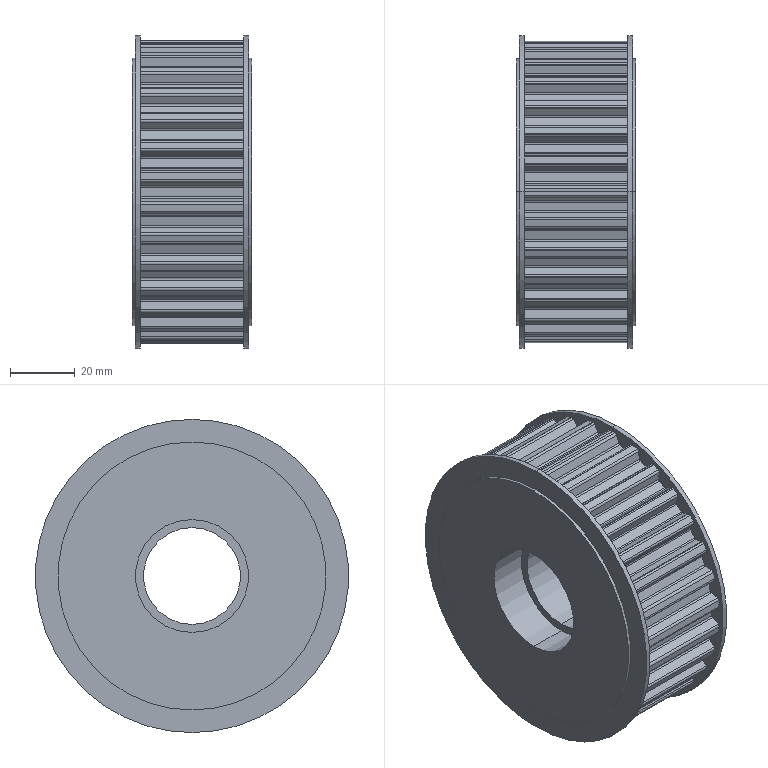Part | SolidWorks | features ICE 6, MirrorPattern 3, Fillet 2, CirPattern 1, Extrusion 1 | 1 solid | 283 faces | box 37 x 97 x 97 mm | volume 204655 mm3 | cylinder 185 | plane 98 | commonest cylinder face diameters 1.2 x70 1.6 x70 93.64 x31 35 x4 83 x4 97 x4